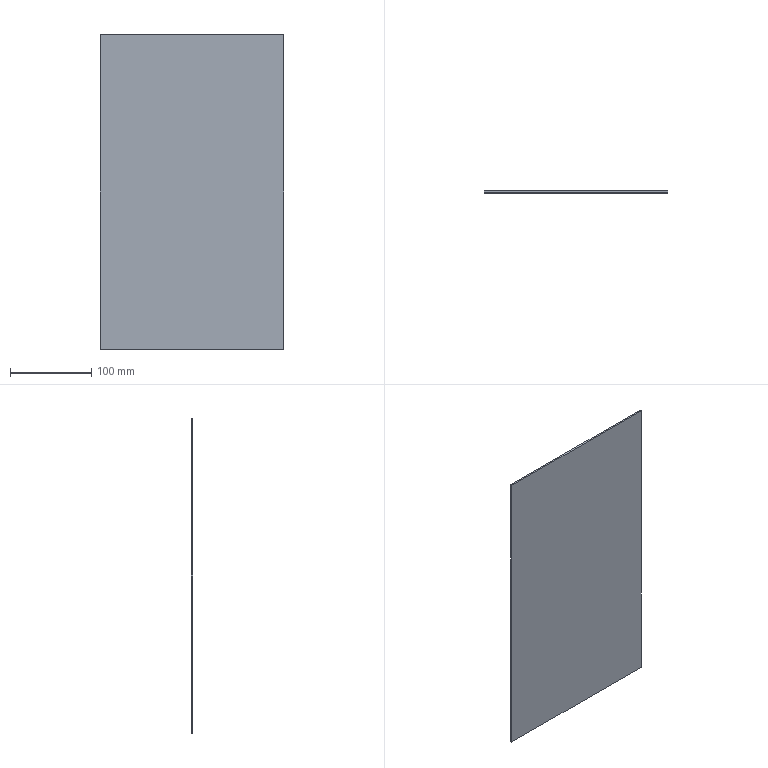Part | STEP file | 1 solid | 6 faces | box 226.259 x 2 x 387.57 mm | volume 175382 mm3 | plane 6
STEP:
#1=CARTESIAN_POINT('',(0.,0.,0.));
#2=DIRECTION('',(0.,0.,1.));
#3=DIRECTION('',(1.,0.,0.));
#4=AXIS2_PLACEMENT_3D('',#1,#2,#3);
#5=CARTESIAN_POINT('',(-81.848,33.164,6.071));
#6=VERTEX_POINT('',#5);
#7=CARTESIAN_POINT('',(-81.848,33.164,393.641));
#8=VERTEX_POINT('',#7);
#9=CARTESIAN_POINT('',(-81.848,33.164,-106.359));
#10=DIRECTION('',(0.,0.,1.));
#11=VECTOR('',#10,1.);
#12=LINE('',#9,#11);
#13=CARTESIAN_POINT('',(-81.848,35.164,-106.359));
#14=DIRECTION('',(1.,0.,0.));
#15=DIRECTION('',(0.,1.,0.));
#16=AXIS2_PLACEMENT_3D('',#13,#14,#15);
#17=PLANE('',#16);
#18=CARTESIAN_POINT('',(-2.,0.));
#19=DIRECTION('',(0.,1.));
#20=VECTOR('',#19,1.);
#21=LINE('',#18,#20);
#22=(GEOMETRIC_REPRESENTATION_CONTEXT(2)PARAMETRIC_REPRESENTATION_CONTEXT()REPRESENTATION_CONTEXT('',''));
#23=DEFINITIONAL_REPRESENTATION('',(#21),#22);
#24=PCURVE('',#17,#23);
#25=CARTESIAN_POINT('',(0.,33.164,0.));
#26=DIRECTION('',(0.,1.,0.));
#27=DIRECTION('',(-1.,0.,0.));
#28=AXIS2_PLACEMENT_3D('',#25,#26,#27);
#29=PLANE('',#28);
#30=CARTESIAN_POINT('',(81.848,-106.359));
#31=DIRECTION('',(0.,1.));
#32=VECTOR('',#31,1.);
#33=LINE('',#30,#32);
#34=(GEOMETRIC_REPRESENTATION_CONTEXT(2)PARAMETRIC_REPRESENTATION_CONTEXT()REPRESENTATION_CONTEXT('',''));
#35=DEFINITIONAL_REPRESENTATION('',(#33),#34);
#36=PCURVE('',#29,#35);
#37=SURFACE_CURVE('',#12,(#24,#36),.PCURVE_S1.);
#38=EDGE_CURVE('',#6,#8,#37,.T.);
#39=ORIENTED_EDGE('',*,*,#38,.T.);
#40=CARTESIAN_POINT('',(-81.848,35.164,393.641));
#41=VERTEX_POINT('',#40);
#42=CARTESIAN_POINT('',(-81.848,35.164,393.641));
#43=DIRECTION('',(0.,-1.,0.));
#44=VECTOR('',#43,1.);
#45=LINE('',#42,#44);
#46=CARTESIAN_POINT('',(0.,500.));
#47=DIRECTION('',(-1.,0.));
#48=VECTOR('',#47,1.);
#49=LINE('',#46,#48);
#50=(GEOMETRIC_REPRESENTATION_CONTEXT(2)PARAMETRIC_REPRESENTATION_CONTEXT()REPRESENTATION_CONTEXT('',''));
#51=DEFINITIONAL_REPRESENTATION('',(#49),#50);
#52=PCURVE('',#17,#51);
#53=CARTESIAN_POINT('',(-144.411,35.164,393.641));
#54=DIRECTION('',(0.,0.,-1.));
#55=DIRECTION('',(-1.,0.,0.));
#56=AXIS2_PLACEMENT_3D('',#53,#54,#55);
#57=PLANE('',#56);
#58=CARTESIAN_POINT('',(-62.563,0.));
#59=DIRECTION('',(0.,-1.));
#60=VECTOR('',#59,1.);
#61=LINE('',#58,#60);
#62=(GEOMETRIC_REPRESENTATION_CONTEXT(2)PARAMETRIC_REPRESENTATION_CONTEXT()REPRESENTATION_CONTEXT('',''));
#63=DEFINITIONAL_REPRESENTATION('',(#61),#62);
#64=PCURVE('',#57,#63);
#65=SURFACE_CURVE('',#45,(#52,#64),.PCURVE_S1.);
#66=EDGE_CURVE('',#41,#8,#65,.T.);
#67=ORIENTED_EDGE('',*,*,#66,.F.);
#68=CARTESIAN_POINT('',(-81.848,35.164,6.071));
#69=VERTEX_POINT('',#68);
#70=CARTESIAN_POINT('',(-81.848,35.164,-106.359));
#71=DIRECTION('',(0.,0.,1.));
#72=VECTOR('',#71,1.);
#73=LINE('',#70,#72);
#74=CARTESIAN_POINT('',(0.,0.));
#75=DIRECTION('',(0.,1.));
#76=VECTOR('',#75,1.);
#77=LINE('',#74,#76);
#78=(GEOMETRIC_REPRESENTATION_CONTEXT(2)PARAMETRIC_REPRESENTATION_CONTEXT()REPRESENTATION_CONTEXT('',''));
#79=DEFINITIONAL_REPRESENTATION('',(#77),#78);
#80=PCURVE('',#17,#79);
#81=CARTESIAN_POINT('',(0.,35.164,0.));
#82=DIRECTION('',(0.,1.,0.));
#83=DIRECTION('',(-1.,0.,0.));
#84=AXIS2_PLACEMENT_3D('',#81,#82,#83);
#85=PLANE('',#84);
#86=CARTESIAN_POINT('',(81.848,-106.359));
#87=DIRECTION('',(0.,1.));
#88=VECTOR('',#87,1.);
#89=LINE('',#86,#88);
#90=(GEOMETRIC_REPRESENTATION_CONTEXT(2)PARAMETRIC_REPRESENTATION_CONTEXT()REPRESENTATION_CONTEXT('',''));
#91=DEFINITIONAL_REPRESENTATION('',(#89),#90);
#92=PCURVE('',#85,#91);
#93=SURFACE_CURVE('',#73,(#80,#92),.PCURVE_S1.);
#94=EDGE_CURVE('',#69,#41,#93,.T.);
#95=ORIENTED_EDGE('',*,*,#94,.F.);
#96=CARTESIAN_POINT('',(-81.848,35.164,6.071));
#97=DIRECTION('',(0.,-1.,0.));
#98=VECTOR('',#97,1.);
#99=LINE('',#96,#98);
#100=CARTESIAN_POINT('',(0.,112.43));
#101=DIRECTION('',(-1.,0.));
#102=VECTOR('',#101,1.);
#103=LINE('',#100,#102);
#104=(GEOMETRIC_REPRESENTATION_CONTEXT(2)PARAMETRIC_REPRESENTATION_CONTEXT()REPRESENTATION_CONTEXT('',''));
#105=DEFINITIONAL_REPRESENTATION('',(#103),#104);
#106=PCURVE('',#17,#105);
#107=CARTESIAN_POINT('',(-144.411,35.164,6.071));
#108=DIRECTION('',(0.,0.,1.));
#109=DIRECTION('',(1.,0.,0.));
#110=AXIS2_PLACEMENT_3D('',#107,#108,#109);
#111=PLANE('',#110);
#112=CARTESIAN_POINT('',(62.563,0.));
#113=DIRECTION('',(0.,-1.));
#114=VECTOR('',#113,1.);
#115=LINE('',#112,#114);
#116=(GEOMETRIC_REPRESENTATION_CONTEXT(2)PARAMETRIC_REPRESENTATION_CONTEXT()REPRESENTATION_CONTEXT('',''));
#117=DEFINITIONAL_REPRESENTATION('',(#115),#116);
#118=PCURVE('',#111,#117);
#119=SURFACE_CURVE('',#99,(#106,#118),.PCURVE_S1.);
#120=EDGE_CURVE('',#69,#6,#119,.T.);
#121=ORIENTED_EDGE('',*,*,#120,.T.);
#122=EDGE_LOOP('',(#39,#67,#95,#121));
#123=FACE_BOUND('',#122,.T.);
#124=ADVANCED_FACE('',(#123),#17,.F.);
#125=CARTESIAN_POINT('',(144.411,33.164,393.641));
#126=VERTEX_POINT('',#125);
#127=CARTESIAN_POINT('',(-144.411,33.164,393.641));
#128=DIRECTION('',(1.,0.,0.));
#129=VECTOR('',#128,1.);
#130=LINE('',#127,#129);
#131=CARTESIAN_POINT('',(0.,-2.));
#132=DIRECTION('',(-1.,0.));
#133=VECTOR('',#132,1.);
#134=LINE('',#131,#133);
#135=(GEOMETRIC_REPRESENTATION_CONTEXT(2)PARAMETRIC_REPRESENTATION_CONTEXT()REPRESENTATION_CONTEXT('',''));
#136=DEFINITIONAL_REPRESENTATION('',(#134),#135);
#137=PCURVE('',#57,#136);
#138=CARTESIAN_POINT('',(144.411,393.641));
#139=DIRECTION('',(-1.,0.));
#140=VECTOR('',#139,1.);
#141=LINE('',#138,#140);
#142=(GEOMETRIC_REPRESENTATION_CONTEXT(2)PARAMETRIC_REPRESENTATION_CONTEXT()REPRESENTATION_CONTEXT('',''));
#143=DEFINITIONAL_REPRESENTATION('',(#141),#142);
#144=PCURVE('',#29,#143);
#145=SURFACE_CURVE('',#130,(#137,#144),.PCURVE_S1.);
#146=EDGE_CURVE('',#8,#126,#145,.T.);
#147=ORIENTED_EDGE('',*,*,#146,.T.);
#148=CARTESIAN_POINT('',(144.411,35.164,393.641));
#149=VERTEX_POINT('',#148);
#150=CARTESIAN_POINT('',(144.411,35.164,393.641));
#151=DIRECTION('',(0.,-1.,0.));
#152=VECTOR('',#151,1.);
#153=LINE('',#150,#152);
#154=CARTESIAN_POINT('',(-288.821,0.));
#155=DIRECTION('',(0.,-1.));
#156=VECTOR('',#155,1.);
#157=LINE('',#154,#156);
#158=(GEOMETRIC_REPRESENTATION_CONTEXT(2)PARAMETRIC_REPRESENTATION_CONTEXT()REPRESENTATION_CONTEXT('',''));
#159=DEFINITIONAL_REPRESENTATION('',(#157),#158);
#160=PCURVE('',#57,#159);
#161=CARTESIAN_POINT('',(144.411,35.164,-106.359));
#162=DIRECTION('',(-1.,0.,0.));
#163=DIRECTION('',(0.,-1.,0.));
#164=AXIS2_PLACEMENT_3D('',#161,#162,#163);
#165=PLANE('',#164);
#166=CARTESIAN_POINT('',(0.,500.));
#167=DIRECTION('',(1.,0.));
#168=VECTOR('',#167,1.);
#169=LINE('',#166,#168);
#170=(GEOMETRIC_REPRESENTATION_CONTEXT(2)PARAMETRIC_REPRESENTATION_CONTEXT()REPRESENTATION_CONTEXT('',''));
#171=DEFINITIONAL_REPRESENTATION('',(#169),#170);
#172=PCURVE('',#165,#171);
#173=SURFACE_CURVE('',#153,(#160,#172),.PCURVE_S1.);
#174=EDGE_CURVE('',#149,#126,#173,.T.);
#175=ORIENTED_EDGE('',*,*,#174,.F.);
#176=CARTESIAN_POINT('',(-144.411,35.164,393.641));
#177=DIRECTION('',(1.,0.,0.));
#178=VECTOR('',#177,1.);
#179=LINE('',#176,#178);
#180=CARTESIAN_POINT('',(0.,0.));
#181=DIRECTION('',(-1.,0.));
#182=VECTOR('',#181,1.);
#183=LINE('',#180,#182);
#184=(GEOMETRIC_REPRESENTATION_CONTEXT(2)PARAMETRIC_REPRESENTATION_CONTEXT()REPRESENTATION_CONTEXT('',''));
#185=DEFINITIONAL_REPRESENTATION('',(#183),#184);
#186=PCURVE('',#57,#185);
#187=CARTESIAN_POINT('',(144.411,393.641));
#188=DIRECTION('',(-1.,0.));
#189=VECTOR('',#188,1.);
#190=LINE('',#187,#189);
#191=(GEOMETRIC_REPRESENTATION_CONTEXT(2)PARAMETRIC_REPRESENTATION_CONTEXT()REPRESENTATION_CONTEXT('',''));
#192=DEFINITIONAL_REPRESENTATION('',(#190),#191);
#193=PCURVE('',#85,#192);
#194=SURFACE_CURVE('',#179,(#186,#193),.PCURVE_S1.);
#195=EDGE_CURVE('',#41,#149,#194,.T.);
#196=ORIENTED_EDGE('',*,*,#195,.F.);
#197=ORIENTED_EDGE('',*,*,#66,.T.);
#198=EDGE_LOOP('',(#147,#175,#196,#197));
#199=FACE_BOUND('',#198,.T.);
#200=ADVANCED_FACE('',(#199),#57,.F.);
#201=CARTESIAN_POINT('',(144.411,33.164,6.071));
#202=VERTEX_POINT('',#201);
#203=CARTESIAN_POINT('',(144.411,33.164,-106.359));
#204=DIRECTION('',(0.,0.,-1.));
#205=VECTOR('',#204,1.);
#206=LINE('',#203,#205);
#207=CARTESIAN_POINT('',(2.,0.));
#208=DIRECTION('',(0.,-1.));
#209=VECTOR('',#208,1.);
#210=LINE('',#207,#209);
#211=(GEOMETRIC_REPRESENTATION_CONTEXT(2)PARAMETRIC_REPRESENTATION_CONTEXT()REPRESENTATION_CONTEXT('',''));
#212=DEFINITIONAL_REPRESENTATION('',(#210),#211);
#213=PCURVE('',#165,#212);
#214=CARTESIAN_POINT('',(-144.411,-106.359));
#215=DIRECTION('',(0.,-1.));
#216=VECTOR('',#215,1.);
#217=LINE('',#214,#216);
#218=(GEOMETRIC_REPRESENTATION_CONTEXT(2)PARAMETRIC_REPRESENTATION_CONTEXT()REPRESENTATION_CONTEXT('',''));
#219=DEFINITIONAL_REPRESENTATION('',(#217),#218);
#220=PCURVE('',#29,#219);
#221=SURFACE_CURVE('',#206,(#213,#220),.PCURVE_S1.);
#222=EDGE_CURVE('',#126,#202,#221,.T.);
#223=ORIENTED_EDGE('',*,*,#222,.T.);
#224=CARTESIAN_POINT('',(144.411,35.164,6.071));
#225=VERTEX_POINT('',#224);
#226=CARTESIAN_POINT('',(144.411,35.164,6.071));
#227=DIRECTION('',(0.,-1.,0.));
#228=VECTOR('',#227,1.);
#229=LINE('',#226,#228);
#230=CARTESIAN_POINT('',(0.,112.43));
#231=DIRECTION('',(1.,0.));
#232=VECTOR('',#231,1.);
#233=LINE('',#230,#232);
#234=(GEOMETRIC_REPRESENTATION_CONTEXT(2)PARAMETRIC_REPRESENTATION_CONTEXT()REPRESENTATION_CONTEXT('',''));
#235=DEFINITIONAL_REPRESENTATION('',(#233),#234);
#236=PCURVE('',#165,#235);
#237=CARTESIAN_POINT('',(288.821,0.));
#238=DIRECTION('',(0.,-1.));
#239=VECTOR('',#238,1.);
#240=LINE('',#237,#239);
#241=(GEOMETRIC_REPRESENTATION_CONTEXT(2)PARAMETRIC_REPRESENTATION_CONTEXT()REPRESENTATION_CONTEXT('',''));
#242=DEFINITIONAL_REPRESENTATION('',(#240),#241);
#243=PCURVE('',#111,#242);
#244=SURFACE_CURVE('',#229,(#236,#243),.PCURVE_S1.);
#245=EDGE_CURVE('',#225,#202,#244,.T.);
#246=ORIENTED_EDGE('',*,*,#245,.F.);
#247=CARTESIAN_POINT('',(144.411,35.164,-106.359));
#248=DIRECTION('',(0.,0.,-1.));
#249=VECTOR('',#248,1.);
#250=LINE('',#247,#249);
#251=CARTESIAN_POINT('',(0.,0.));
#252=DIRECTION('',(0.,-1.));
#253=VECTOR('',#252,1.);
#254=LINE('',#251,#253);
#255=(GEOMETRIC_REPRESENTATION_CONTEXT(2)PARAMETRIC_REPRESENTATION_CONTEXT()REPRESENTATION_CONTEXT('',''));
#256=DEFINITIONAL_REPRESENTATION('',(#254),#255);
#257=PCURVE('',#165,#256);
#258=CARTESIAN_POINT('',(-144.411,-106.359));
#259=DIRECTION('',(0.,-1.));
#260=VECTOR('',#259,1.);
#261=LINE('',#258,#260);
#262=(GEOMETRIC_REPRESENTATION_CONTEXT(2)PARAMETRIC_REPRESENTATION_CONTEXT()REPRESENTATION_CONTEXT('',''));
#263=DEFINITIONAL_REPRESENTATION('',(#261),#262);
#264=PCURVE('',#85,#263);
#265=SURFACE_CURVE('',#250,(#257,#264),.PCURVE_S1.);
#266=EDGE_CURVE('',#149,#225,#265,.T.);
#267=ORIENTED_EDGE('',*,*,#266,.F.);
#268=ORIENTED_EDGE('',*,*,#174,.T.);
#269=EDGE_LOOP('',(#223,#246,#267,#268));
#270=FACE_BOUND('',#269,.T.);
#271=ADVANCED_FACE('',(#270),#165,.F.);
#272=CARTESIAN_POINT('',(-144.411,33.164,6.071));
#273=DIRECTION('',(-1.,0.,0.));
#274=VECTOR('',#273,1.);
#275=LINE('',#272,#274);
#276=CARTESIAN_POINT('',(0.,-2.));
#277=DIRECTION('',(-1.,0.));
#278=VECTOR('',#277,1.);
#279=LINE('',#276,#278);
#280=(GEOMETRIC_REPRESENTATION_CONTEXT(2)PARAMETRIC_REPRESENTATION_CONTEXT()REPRESENTATION_CONTEXT('',''));
#281=DEFINITIONAL_REPRESENTATION('',(#279),#280);
#282=PCURVE('',#111,#281);
#283=CARTESIAN_POINT('',(144.411,6.071));
#284=DIRECTION('',(1.,0.));
#285=VECTOR('',#284,1.);
#286=LINE('',#283,#285);
#287=(GEOMETRIC_REPRESENTATION_CONTEXT(2)PARAMETRIC_REPRESENTATION_CONTEXT()REPRESENTATION_CONTEXT('',''));
#288=DEFINITIONAL_REPRESENTATION('',(#286),#287);
#289=PCURVE('',#29,#288);
#290=SURFACE_CURVE('',#275,(#282,#289),.PCURVE_S1.);
#291=EDGE_CURVE('',#202,#6,#290,.T.);
#292=ORIENTED_EDGE('',*,*,#291,.T.);
#293=ORIENTED_EDGE('',*,*,#120,.F.);
#294=CARTESIAN_POINT('',(-144.411,35.164,6.071));
#295=DIRECTION('',(-1.,0.,0.));
#296=VECTOR('',#295,1.);
#297=LINE('',#294,#296);
#298=CARTESIAN_POINT('',(0.,0.));
#299=DIRECTION('',(-1.,0.));
#300=VECTOR('',#299,1.);
#301=LINE('',#298,#300);
#302=(GEOMETRIC_REPRESENTATION_CONTEXT(2)PARAMETRIC_REPRESENTATION_CONTEXT()REPRESENTATION_CONTEXT('',''));
#303=DEFINITIONAL_REPRESENTATION('',(#301),#302);
#304=PCURVE('',#111,#303);
#305=CARTESIAN_POINT('',(144.411,6.071));
#306=DIRECTION('',(1.,0.));
#307=VECTOR('',#306,1.);
#308=LINE('',#305,#307);
#309=(GEOMETRIC_REPRESENTATION_CONTEXT(2)PARAMETRIC_REPRESENTATION_CONTEXT()REPRESENTATION_CONTEXT('',''));
#310=DEFINITIONAL_REPRESENTATION('',(#308),#309);
#311=PCURVE('',#85,#310);
#312=SURFACE_CURVE('',#297,(#304,#311),.PCURVE_S1.);
#313=EDGE_CURVE('',#225,#69,#312,.T.);
#314=ORIENTED_EDGE('',*,*,#313,.F.);
#315=ORIENTED_EDGE('',*,*,#245,.T.);
#316=EDGE_LOOP('',(#292,#293,#314,#315));
#317=FACE_BOUND('',#316,.T.);
#318=ADVANCED_FACE('',(#317),#111,.F.);
#319=ORIENTED_EDGE('',*,*,#94,.T.);
#320=ORIENTED_EDGE('',*,*,#195,.T.);
#321=ORIENTED_EDGE('',*,*,#266,.T.);
#322=ORIENTED_EDGE('',*,*,#313,.T.);
#323=EDGE_LOOP('',(#319,#320,#321,#322));
#324=FACE_BOUND('',#323,.T.);
#325=ADVANCED_FACE('',(#324),#85,.T.);
#326=ORIENTED_EDGE('',*,*,#38,.F.);
#327=ORIENTED_EDGE('',*,*,#291,.F.);
#328=ORIENTED_EDGE('',*,*,#222,.F.);
#329=ORIENTED_EDGE('',*,*,#146,.F.);
#330=EDGE_LOOP('',(#326,#327,#328,#329));
#331=FACE_BOUND('',#330,.T.);
#332=ADVANCED_FACE('',(#331),#29,.F.);
#333=CLOSED_SHELL('',(#124,#200,#271,#318,#325,#332));
#334=MANIFOLD_SOLID_BREP('',#333);
#335=(LENGTH_UNIT()NAMED_UNIT(*)SI_UNIT(.MILLI.,.METRE.));
#336=UNCERTAINTY_MEASURE_WITH_UNIT(LENGTH_MEASURE(0.0000001),#335,'','');
#337=(NAMED_UNIT(*)PLANE_ANGLE_UNIT()SI_UNIT($,.RADIAN.));
#338=(NAMED_UNIT(*)SI_UNIT($,.STERADIAN.)SOLID_ANGLE_UNIT());
#339=(GEOMETRIC_REPRESENTATION_CONTEXT(3)GLOBAL_UNCERTAINTY_ASSIGNED_CONTEXT((#336))GLOBAL_UNIT_ASSIGNED_CONTEXT((#335,#337,#338))REPRESENTATION_CONTEXT('',''));
#340=ADVANCED_BREP_SHAPE_REPRESENTATION('',(#4,#334),#339);